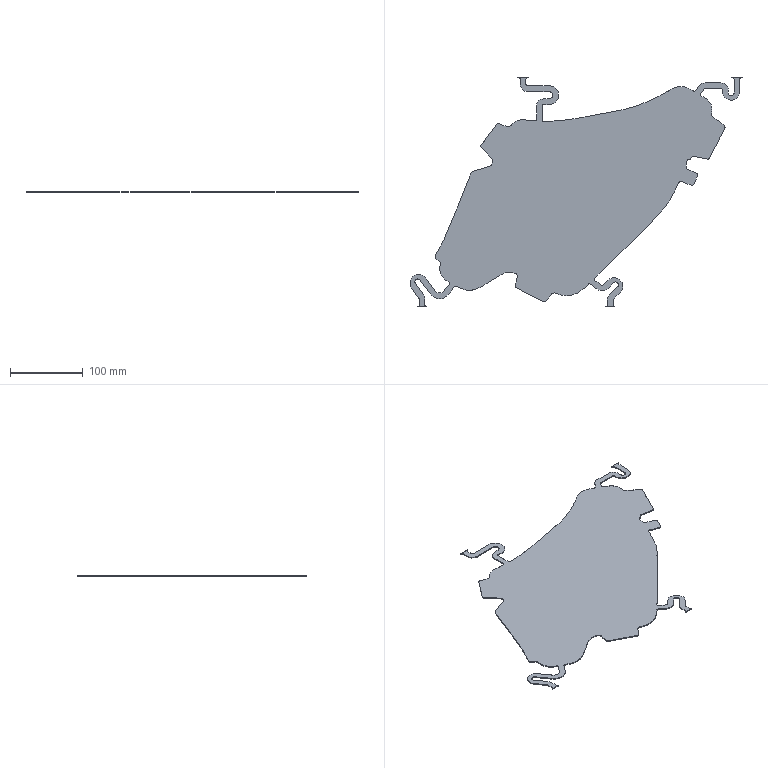Part | STEP file | gslz 2016.10.28-13_id230_x_t | 1 solid | 204 faces | box 457.141 x 316.496 x 1.25 mm | volume 89393 mm3 | plane 110 | cylinder 94 | commonest cylinder face diameters 4 x35 6 x13 8 x6 10 x6 20 x6 24 x4